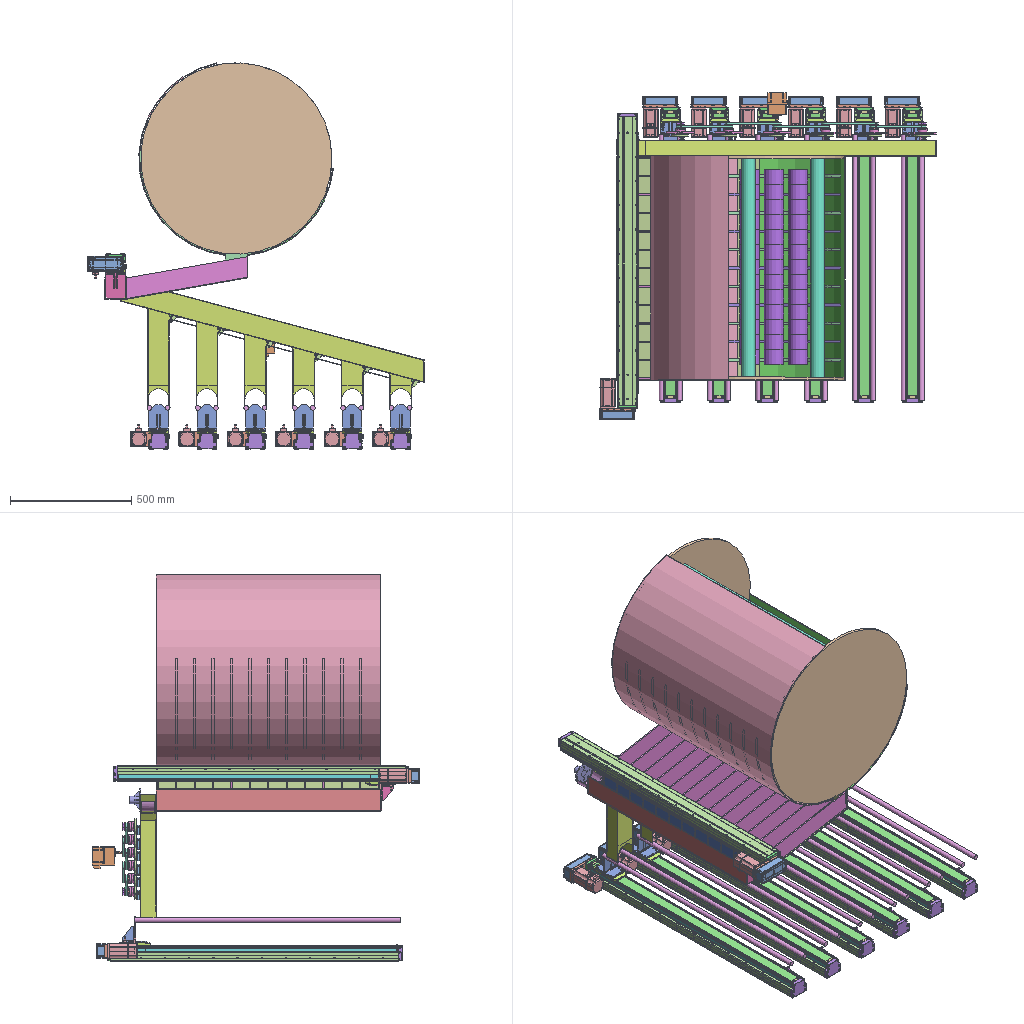Assembly | NX | 55 different items | 545 placed | box 1392 x 1351 x 1595 mm
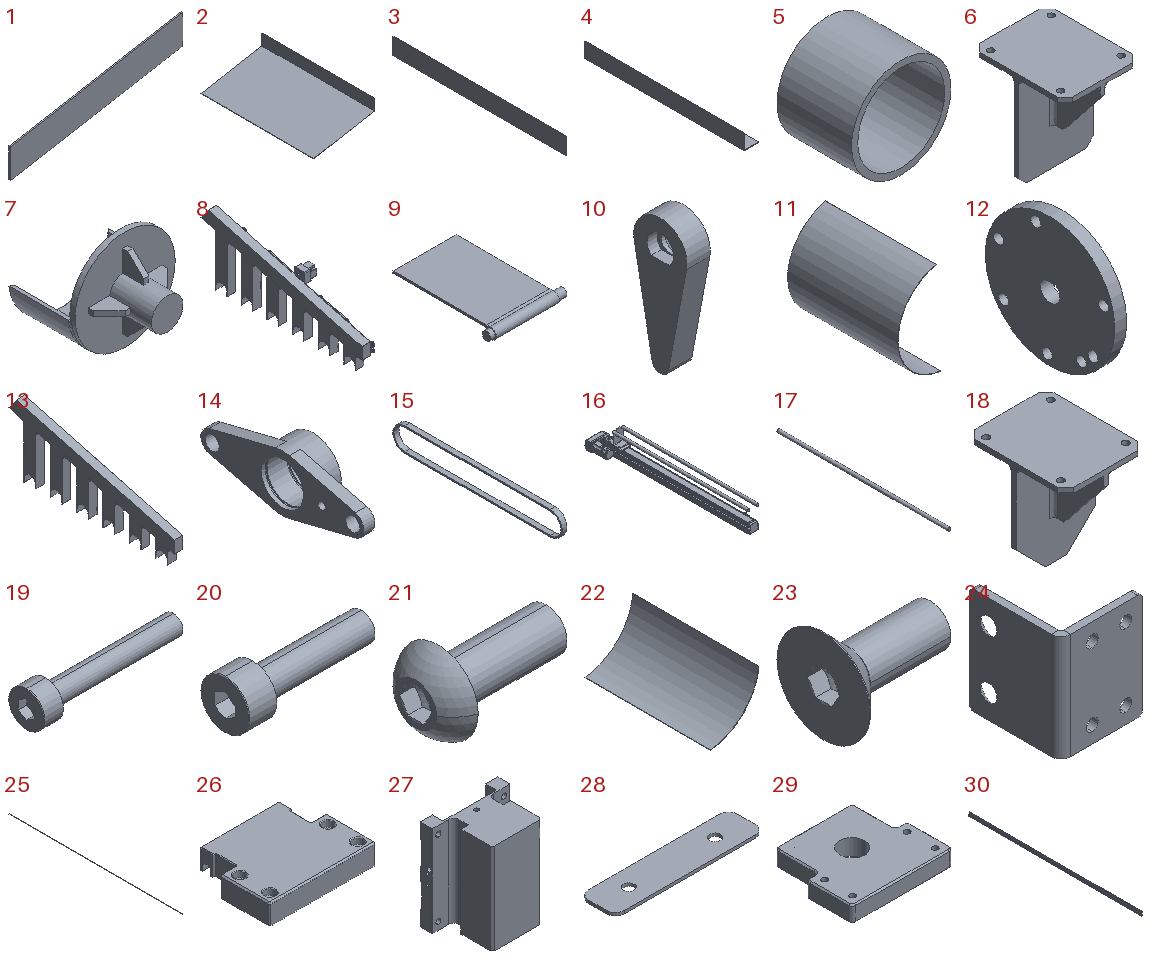Parts list (item | quantity | parent item | size | volume | features):
1 | x13 | in 55 | 500 x 5 x 173.163 mm | 212500 mm3 | features DATUM_CSYS 1, EXTRUDE 1, LINKED_CURVE 1
2 | x1 | in 55 | 503 x 926 x 181.118 mm | 1667441 mm3 | features DATUM_CSYS 1, EXTRUDE 1, LINKED_CURVE 1
3 | x1 | in 55 | 3 x 926 x 90 mm | 250020 mm3 | features DATUM_CSYS 1, EXTRUDE 1, LINKED_CURVE 1
4 | x1 | in 55 | 85 x 926 x 88 mm | 472260 mm3 | features DATUM_CSYS 1, EXTRUDE 1, LINKED_CURVE 1, MOVE_FACE 1
5 | x39 | - | 80 x 60 x 80 mm | 70686 mm3 | features DATUM_CSYS 2, EXTRUDE 1, SKETCH 1
6 | x1 | - | 80 x 100 x 105 mm | 89889 mm3 | features FILLET_WELD 5, FSET 5, EXTRUDE 3, DATUM_CSYS 2, UNITE 2, CHAMFER 1, SKETCH 1
7 | x1 | - | 95.064 x 103 x 95.3 mm | 92637 mm3 | features EXTRUDE 7, CHAMFER 5, EXTRACT_FACE 4, EXTRACT_STRING 4, Instance Feature 3, DATUM_CSYS 2, FSET 2, DIVIDE_FACE 1, FILLET_WELD 1, Pattern Feature 1, SKETCH 1, WELD_GROOVE 1
8 | x1 | - | - | 2656651 mm3 | features EXTRUDE 30, EXTRACT_STRING 18, Instance Feature 16, DATUM_CSYS 14, EXTRACT_FACE 14, SKETCH 9, BREP 7, skf_bearing_4200_atn9_2_1 5, HOLE PACKAGE 3, Pattern Feature 3, FSET 2, MOVE_FACE 2, OFFSET_REGION 2, RECT_GROOVE 2, SIMPLE HOLE 2, SYMBOLIC_THREAD 2, CSUNK_HOLE 1, DIVIDE_FACE 1, FILLET_WELD 1, LINE 1, LINKED_CURVE 1, Mirror Feature 1, SHELL 1, WELD_GROOVE 1
9 | x6 | in 8 | 74 x 100 x 10 mm | 16601 mm3 | features EXTRUDE 4, DATUM_CSYS 2, FSET 2, FILLET_WELD 1, HOLE PACKAGE 1, SIMPLE HOLE 1, SKETCH 1, SYMBOLIC_THREAD 1, WELD_GROOVE 1
10 | x6 | in 8 | 7 x 16 x 40.5 mm | 2685 mm3 | features DATUM_CSYS 2, EXTRUDE 2, SKETCH 2, CSUNK_HOLE 1, HOLE PACKAGE 1
11 | x1 | - | 358 x 926 x 795.299 mm | 3153696 mm3 | features DATUM_CSYS 2, EXTRUDE 1, SKETCH 1
12 | x6 | in 8 | 6 x 65.544 x 65.544 mm | 18977 mm3 | features EXTRUDE 8, EXTRACT_FACE 6, EXTRACT_STRING 6, Instance Feature 5, DATUM_CSYS 2, SKETCH 2, HOLE PACKAGE 1, LINKED_CURVE 1, Pattern Feature 1, SIMPLE HOLE 1, SYMBOLIC_THREAD 1
13 | x1 | in 8 | 66 x 1255 x 510.77 mm | 1518508 mm3 | features EXTRUDE 13, EXTRACT_STRING 12, Instance Feature 10, EXTRACT_FACE 6, DATUM_CSYS 3, Pattern Feature 2, SKETCH 2, DIVIDE_FACE 1, LINE 1, SHELL 1
14 | x6 | in 8 | 22 x 116 x 40 mm | 25110 mm3 | features DATUM_CSYS 3, EXTRACT_FACE 2, EXTRUDE 2, RECT_GROOVE 2, Instance Feature 1, Mirror Feature 1, SKETCH 1
15 | x5 | in 8 | 7 x 241.055 x 34 mm | 7205 mm3 | features DATUM_CSYS 2, EXTRUDE 1, SKETCH 1
16 | x6 | - | 163 x 1265 x 183 mm | 4732043 mm3 | features BREP 20, FILLET_WELD 5, FSET 5, DATUM_CSYS 3, EXTRUDE 3, MOVE_FACE 2, UNITE 2, CHAMFER 1, CYLINDER 1, SKETCH 1
17 | x12 | in 16 | 20 x 1100 x 20 mm | 345575 mm3 | features CYLINDER 1, DATUM_CSYS 1
18 | x6 | in 16 | 80 x 100 x 105 mm | 85942 mm3 | features FILLET_WELD 5, FSET 5, EXTRUDE 3, DATUM_CSYS 2, MOVE_FACE 2, UNITE 2, CHAMFER 1, SKETCH 1
19 | x28 | in 39 | 23 x 5.5 x 5.5 mm | 205.277 mm3 | features BREP 1
20 | x56 | in 39 | 20 x 7 x 7 mm | 338.493 mm3 | features BREP 1
21 | x56 | in 39 | 9.65 x 5.7 x 5.7 mm | 80.89 mm3 | features BREP 1
22 | x1 | - | 355.98 x 926 x 360.442 mm | 1514546 mm3 | features DATUM_CSYS 2, EXTRUDE 1, SKETCH 1
23 | x28 | in 39 | 8 x 6.72 x 6.72 mm | 75.41 mm3 | features BREP 1
24 | x21 | in 39 | 17 x 19 x 22 mm | 1032 mm3 | features BREP 1
25 | x14 | in 39 | 3.5 x 1190 x 0.5 mm | 2082 mm3 | features BREP 1
26 | x7 | in 39 | 80 x 63 x 15 mm | 64331 mm3 | features BREP 1
27 | x7 | in 39 | 77 x 58.5 x 90 mm | 226151 mm3 | features BREP 1
28 | x14 | in 39 | 50 x 12 x 1 mm | 571.917 mm3 | features BREP 1
29 | x7 | in 39 | 81 x 71.5 x 13 mm | 60726 mm3 | features BREP 1
30 | x14 | in 39 | 8.5 x 1190 x 27 mm | 74453 mm3 | features BREP 1
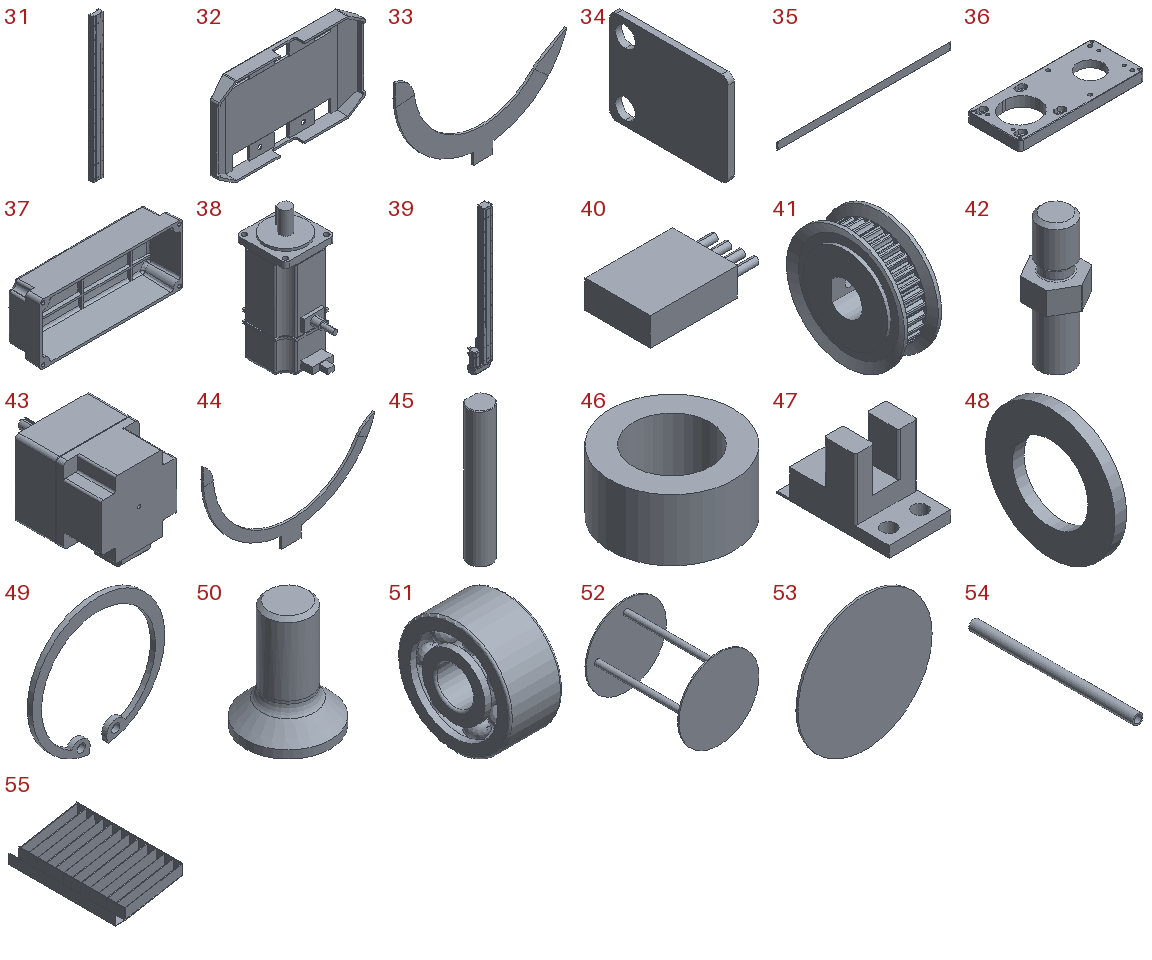31 | x7 | in 39 | 82 x 38 x 1190 mm | 3089762 mm3 | features BREP 1
32 | x7 | in 39 | 135 x 11.5 x 81 mm | 22124 mm3 | features BREP 1
33 | x5 | - | 781.576 x 10 x 500 mm | 886213 mm3 | features DATUM_CSYS 2, DIVIDE_FACE 1, EXTRUDE 1, SKETCH 1
34 | x7 | in 39 | 1 x 19 x 15 mm | 268.057 mm3 | features BREP 1
35 | x7 | in 39 | 1190 x 0.2 x 50 mm | 11880 mm3 | features BREP 1
36 | x7 | in 39 | 146.5 x 62 x 12 mm | 74103 mm3 | features BREP 1
37 | x7 | in 39 | 146.5 x 34.5 x 62 mm | 53198 mm3 | features BREP 1
38 | x7 | in 39 | 64 x 92 x 154.5 mm | 181603 mm3 | features BREP 1
39 | x7 | in 16 | 162 x 101.5 x 1265 mm | 3954942 mm3 | features BREP 20
40 | x21 | in 39 | 21 x 12 x 5.2 mm | 1028 mm3 | features BREP 1
41 | x12 | in 8 | 11 x 35 x 35 mm | 6439 mm3 | features OFFSET_REGION 2, BREP 1
42 | x6 | in 8 | 8 x 9.2 x 23 mm | 695.67 mm3 | features BREP 1
43 | x1 | in 8 | 80 x 123 x 91 mm | 559615 mm3 | features BREP 1
44 | x6 | - | 781.576 x 10 x 500 mm | 527562 mm3 | features DATUM_CSYS 2, DIVIDE_FACE 1, EXTRUDE 1, SKETCH 1
45 | x6 | in 8 | 10 x 10 x 58 mm | 4439 mm3 | features MOVE_FACE 2, BREP 1
46 | x12 | in 8 | 16 x 16 x 8 mm | 980.177 mm3 | features BREP 1
47 | x21 | in 39 | 13.8 x 25 x 16.25 mm | 2130 mm3 | features BREP 1
48 | x1 | - | 1.6 x 18 x 18 mm | 268.606 mm3 | features BREP 1
49 | x12 | in 8 | 32.1 x 1.2 x 31.887 mm | 256.127 mm3 | features BREP 1
50 | x6 | in 8 | 9.43 x 9.43 x 12 mm | 313.297 mm3 | features BREP 1
51 | x6 | in 8 | 14 x 30 x 30 mm | 6245 mm3 | features skf_bearing_4200_atn9_2_1 5
52 | x1 | - | 790 x 926 x 790 mm | 16116597 mm3 | features DATUM_CSYS 4, EXTRUDE 2, SKETCH 2
53 | x2 | in 52 | 790 x 12 x 790 mm | 5882004 mm3 | features DATUM_CSYS 2, EXTRUDE 1, SKETCH 1
54 | x4 | in 52 | 56 x 902 x 56 mm | 1088147 mm3 | features DATUM_CSYS 2, EXTRUDE 1, SKETCH 1
55 | x1 | - | 591 x 926 x 181.163 mm | 5152221 mm3 | features DATUM_CSYS 4, EXTRUDE 4, LINKED_CURVE 4, MOVE_FACE 1
Mates (type | each side: item.copy, entity, surface, feature):
In the top assembly
Fix | assembly component | 5 times
Bond | 33.1 component | assembly component | 5 times
LinearPattern | assembly axis | assembly csys | assembly csys | assembly csys | assembly csys | assembly csys | 2 times
Bond | 5.1 component | assembly component | 39 times
Linear2dPattern | assembly axis | assembly axis | assembly csys | assembly csys | assembly csys | assembly csys | assembly csys | assembly csys | assembly csys | assembly csys | assembly csys | assembly csys | assembly csys | assembly csys | assembly csys | assembly csys | assembly csys | assembly csys | assembly csys | assembly csys | assembly csys | assembly csys | assembly csys | assembly csys | assembly csys | assembly csys | assembly csys | assembly csys | assembly csys | assembly csys | assembly csys | assembly csys | assembly csys | assembly csys | assembly csys | assembly csys | assembly csys | assembly csys | assembly csys | assembly csys | assembly csys
Fix | 33.1 component
Bond | 44.1 component | assembly component | 7 times
LinearPattern | assembly axis | assembly csys | assembly csys
Distance | 44.1 face plane Divide Face(4) | 33.1 face plane Divide Face(4)
Touch | 44.1 face cylinder Extrude(2) | 33.1 face cylinder Extrude(2)
Touch | 44.1 face plane Extrude(2) | 33.1 face plane Extrude(2)
Touch | 11.1 face cylinder Extrude(2) | 33.1 face cylinder Extrude(2)
Touch | 11.1 edge | 33.1 face plane Extrude(2)
Center22 | 11.1 face plane Extrude(2) | 11.1 face plane Extrude(2) | 33.1 face plane Divide Face(4) | 33.1 face plane Divide Face(4)
Touch | 22.1 face cylinder Extrude(2) | 33.1 face cylinder Extrude(2)
Touch | 22.1 edge | 33.1 face plane Extrude(2)
Touch | 22.1 face plane Extrude(2) | 11.1 face plane Extrude(2)
Touch | 53.1 face cylinder Extrude(2) | 33.1 face cylinder Extrude(2)
Touch | 53.1 face plane Extrude(2) | 11.1 face plane Extrude(2)
Touch | 54.1 face cylinder Extrude(2) | assembly plane
Touch | 2.1 face plane Extrude(4) | 33.1 face plane Extrude(2)
Touch | 2.1 face plane Extrude(4) | 22.1 edge
Center22 | 2.1 face plane Extrude(4) | 2.1 face plane Extrude(4) | 33.1 face plane Divide Face(4) | 33.1 face plane Divide Face(4)
Touch | 6.1 face plane Extrude(2) | 27.1 face plane Body(1)
Touch | 6.1 face cylinder Extrude(2) | 27.1 face cylinder Body(1) | 2 times
Center22 | 6.1 face plane Extrude(2) | 6.1 face plane Extrude(2) | 4.1 face plane Extrude(3) | 3.1 face plane Extrude(3)
Distance | 6.1 face plane Extrude(3) | 4.1 face plane Extrude(3)
Touch | 6.1 face plane Extrude(3) | 4.1 face plane Extrude(3)
Distance | 7.1 face plane Extrude(2) | 4.1 face plane Extrude(3)
Center12 | 3.1 face plane Extrude(3) | 4.1 face plane Extrude(3) | 7.1 face cylinder Extrude(7)
Parallel | 7.1 face plane Pattern Feature [Circular] (6) / Instance[1][0] | 4.1 face plane Extrude(3)
Distance | 7.1 point | 4.1 face plane Extrude(3)
Touch | 13.1 face plane Extrude(3) | 2.1 face plane Extrude(4)
Parallel | 13.1 face plane Extrude(3) | assembly plane
Touch | 13.1 face plane Extrude(3) | 7.1 face cylinder Extrude(7) | 2 times
Center22 | 17.1 face cylinder Cylinder(1) | 17.1 face cylinder Cylinder(1) | 13.1 face plane Extrude(3) | 13.1 face plane Extrude(3)
Distance | 18.1 face plane Extrude(3) | 13.1 face plane Extrude(3) | 2 times
Bond | 16.1 component | assembly component | 6 times
LinearPattern | assembly axis | assembly csys | assembly csys | assembly csys | assembly csys | assembly csys | assembly csys
In subassembly 8
Touch | 10.1 face cylinder Extrude(4) | 9.1 face cylinder Extrude(4)
Touch | 10.1 face plane Extrude(4) | 9.1 face plane Extrude(5) | 2 times
Touch | 50.1 face cylinder Body(1) | 9.1 face cylinder M5 x 0.8 Threaded Hole(10)
Touch | 50.1 face cone Body(1) | 10.1 face cone Ø5.5 Countersunk Hole(5)
Touch | 9.1 face cylinder Extrude(4) | 13.1 face cylinder Extrude(5)
Center22 | 9.1 face plane Extrude(2) | 9.1 face plane Extrude(2) | 13.1 face plane Divide Face(17) | 13.1 face plane Divide Face(17)
Parallel | 9.1 face plane Extrude(3) | 13.1 face plane Shell(4)
Fix | 13.1 component
Bond | 10.1 component | 8.1 component | 6 times
Bond | 50.1 component | 8.1 component | 6 times
Bond | 9.1 component | 8.1 component | 6 times
CommonOffsetTransform | 8.2 csys | 8.2 csys | 8.2 csys | 8.2 csys | 8.2 csys | 8.2 csys | 8.2 csys | 8.2 csys | 8.2 csys | 8.2 csys | 8.2 csys | 8.2 csys | 4 times
Bond | 8.1 component | 8.1 component | 8.1 component | 8.1 component | 8.1 component | 8.1 component | 13.1 component | 4 times
Touch | 42.1 face cylinder Body(1) | 12.1 face cylinder M6 x 1.0 Threaded Hole(5) | 6 times
Touch | 42.1 face plane Body(1) | 12.1 face plane Extrude(3) | 6 times
Touch | 12.1 plane | 10.1 plane | 2 times
Distance | 12.1 plane | 10.1 plane
Touch | 45.1 face plane Body(1) | 12.1 face plane Extrude(4) | 6 times
Touch | 45.1 face cylinder Body(1) | 12.1 face cylinder Extrude(4) | 6 times
Touch | 46.1 face cylinder Body(1) | 12.1 face cylinder Extrude(4) | 12 times
Touch | 46.1 face plane Body(1) | 12.1 face plane Extrude(3) | 6 times
Touch | 51.1 face cylinder skf_bearing_4200_atn9_2_1(2) | 14.1 face cylinder Extrude(3) | 6 times
Touch | 49.1 face plane Body(1) | 14.1 face plane Rectangular Groove(5) | 6 times
Touch | 49.1 face cylinder Body(1) | 14.1 face cylinder Rectangular Groove(5)
Touch | 51.1 face plane skf_bearing_4200_atn9_2_1(2) | 49.1 face plane Body(1) | 6 times
Touch | 49.1 face plane Body(1) | 51.1 face plane skf_bearing_4200_atn9_2_1(2) | 6 times
Touch | 49.1 face cylinder Body(1) | 14.1 face cylinder Mirror Feature(6)
Touch | 14.1 face cylinder Extrude(3) | 45.1 face cylinder Body(1)
Touch | 51.1 face plane skf_bearing_4200_atn9_2_1(1) | 46.1 face plane Body(1) | 6 times
Touch | 46.1 face plane Body(1) | 51.1 face plane skf_bearing_4200_atn9_2_1(1) | 6 times
Touch | 41.1 face plane Body(1) | 41.1 face plane Body(1) | 12 times
Touch | 41.1 face cylinder Body(1) | 41.1 face cylinder Body(1) | 6 times
Touch | 41.1 face cylinder Body(1) | 45.1 face cylinder Body(1) | 6 times
Touch | 41.1 face plane Body(1) | 45.1 face plane Body(1) | 6 times
Touch | 41.1 face plane Body(1) | 46.1 face plane Body(1) | 6 times
Touch | 45.1 face plane Body(1) | 12.1 face plane Extrude(3) | 6 times
Parallel | 14.1 plane | 8.2 plane
Bond | 14.1 component | 8.1 component | 6 times
Touch | 49.1 face cylinder Body(1) | 51.1 face cylinder skf_bearing_4200_atn9_2_1(2) | 10 times
Touch | 51.1 face cylinder skf_bearing_4200_atn9_2_1(2) | 45.1 face cylinder Body(1) | 5 times
Angle | 12.1 plane | 10.1 plane | 5 times
Touch | 43.1 | 45.1 face cylinder Body(1)
Parallel | 43.1 | 8.2 plane
Touch | 43.1 | 45.1 face plane Body(1)
Touch | 15.1 | 41.1 face cylinder Body(1) | 10 times
Touch | 15.1 | 41.1 face plane Body(1) | 5 times
In subassembly 16
Touch | 18.1 face cylinder Extrude(2) | 27.1 face cylinder Body(1) | 2 times
Touch | 18.1 face plane Extrude(2) | 27.1 face plane Body(1)
Touch | 18.1 face plane Extrude(2) | 16.2 plane
Touch | 18.1 face plane Extrude(3) | 16.2 plane
Center12 | 18.1 face plane Extrude(2) | 18.1 face plane Extrude(2) | 16.2 plane
Touch | 17.1 face cylinder Cylinder(1) | 18.1 face plane Chamfer(5)
Touch | 17.1 | 18.1 face plane Chamfer(5)
Distance | 17.1 face cylinder Cylinder(1) | 17.1
Touch | 17.1 face plane Cylinder(1) | 17.1
Center12 | 17.1 | 17.1 face cylinder Cylinder(1) | 16.2 plane
Touch | 17.1 face plane Cylinder(1) | 18.1 face plane Extrude(3)
In subassembly 39
Bond | 32.1 component | 27.1 component | 23.1 component | 23.1 component | 23.1 component | 23.1 component | 34.1 component
Bond | 26.1 component | 21.1 component | 20.1 component | 19.1 component | 24.1 component | 38.1 component | 25.1 component | 30.1 component | 28.1 component | 21.1 component | 20.1 component | 40.1 component | 31.1 component | 24.1 component | 25.1 component | 30.1 component | 28.1 component | 29.1 component | 21.1 component | 21.1 component | 20.1 component | 20.1 component | 24.1 component | 21.1 component | 21.1 component | 20.1 component | 47.1 component | 37.1 component | 40.1 component | 36.1 component | 21.1 component | 21.1 component | 20.1 component | 19.1 component | 47.1 component | 40.1 component | 20.1 component | 19.1 component | 47.1 component | 20.1 component | 19.1 component | 35.1 component
Fix | 37.1 component
Distance | 27.1 | 30.1 | 2 times
Distance | 32.1 | 29.1
In subassembly 52
Touch | 53.1 face plane Extrude(2) | 54.1 face plane Extrude(2) | 2 times
Distance | 54.1 face cylinder Extrude(2) | 52.1 plane
Touch | 53.1 face cylinder Extrude(2) | 52.1 axis | 2 times
Center12 | 53.1 face plane Extrude(2) | 53.1 face plane Extrude(2) | 52.1 plane
Fix | 52.2 component
Bond | 54.1 component | 52.2 component | 4 times
CircularPattern | 52.1 axis | 52.1 csys | 52.1 csys | 52.1 csys | 52.1 csys
Touch | 54.1 face cylinder Extrude(2) | 52.1 plane
In subassembly 55
Fix | 55.1 component
Bond | 1.1 component | 55.1 component | 13 times
LinearPattern | 55.2 axis | 55.2 csys | 55.2 csys | 55.2 csys | 55.2 csys | 55.2 csys | 55.2 csys | 55.2 csys | 55.2 csys | 55.2 csys | 55.2 csys | 55.2 csys | 55.2 csys | 55.2 csys